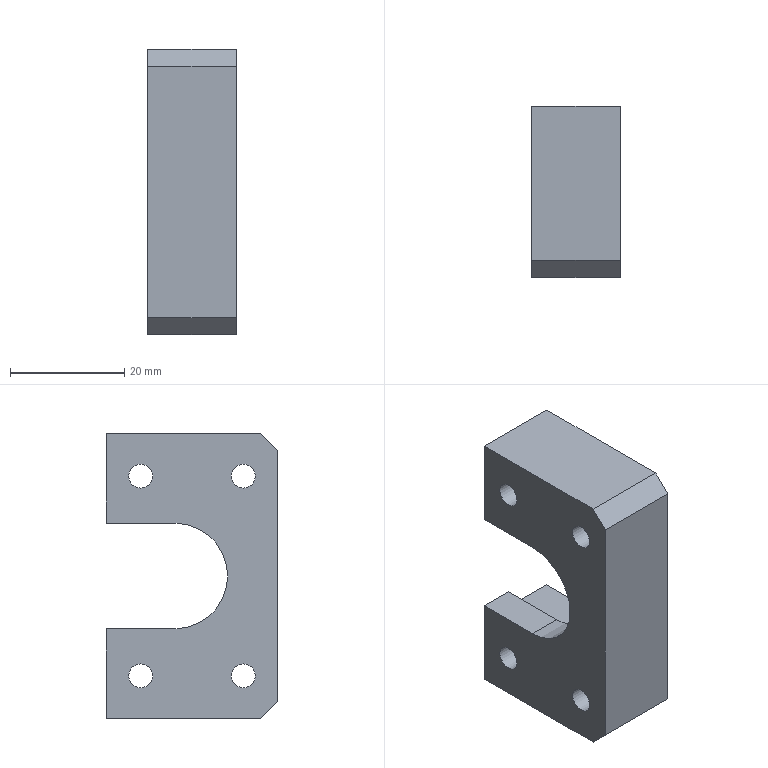Part | NX | 1 solid | 20 faces | box 15.5 x 30 x 50 mm | volume 14931 mm3 | plane 14 | cylinder 6 | commonest cylinder face diameters 4.2 x4 18.5 x1 25 x1
STEP:
#1=CARTESIAN_POINT('',(6.,3.,-9.25));
#2=VERTEX_POINT('',#1);
#3=CARTESIAN_POINT('',(6.,3.,9.25));
#4=VERTEX_POINT('',#3);
#5=CARTESIAN_POINT('',(6.,3.,0.));
#6=DIRECTION('',(1.,0.,0.));
#7=DIRECTION('',(0.,0.,-1.));
#8=AXIS2_PLACEMENT_3D('',#5,#6,#7);
#9=CIRCLE('',#8,9.25);
#10=EDGE_CURVE('',#2,#4,#9,.F.);
#11=ORIENTED_EDGE('',*,*,#10,.F.);
#12=CARTESIAN_POINT('',(0.,3.,-9.25));
#13=VERTEX_POINT('',#12);
#14=CARTESIAN_POINT('',(-4.5,3.,-9.25));
#15=DIRECTION('',(1.,0.,0.));
#16=VECTOR('',#15,1000.);
#17=LINE('',#14,#16);
#18=EDGE_CURVE('',#13,#2,#17,.T.);
#19=ORIENTED_EDGE('',*,*,#18,.F.);
#20=CARTESIAN_POINT('',(0.,3.,9.25));
#21=VERTEX_POINT('',#20);
#22=CARTESIAN_POINT('',(0.,3.,0.));
#23=DIRECTION('',(1.,0.,0.));
#24=DIRECTION('',(0.,0.,-1.));
#25=AXIS2_PLACEMENT_3D('',#22,#23,#24);
#26=CIRCLE('',#25,9.25);
#27=EDGE_CURVE('',#21,#13,#26,.T.);
#28=ORIENTED_EDGE('',*,*,#27,.F.);
#29=CARTESIAN_POINT('',(-4.5,3.,9.25));
#30=DIRECTION('',(1.,0.,0.));
#31=VECTOR('',#30,1000.);
#32=LINE('',#29,#31);
#33=EDGE_CURVE('',#21,#4,#32,.T.);
#34=ORIENTED_EDGE('',*,*,#33,.T.);
#35=EDGE_LOOP('',(#11,#19,#28,#34));
#36=FACE_BOUND('',#35,.T.);
#37=CARTESIAN_POINT('',(-4.5,3.,0.));
#38=DIRECTION('',(1.,0.,0.));
#39=DIRECTION('',(0.,0.,-1.));
#40=AXIS2_PLACEMENT_3D('',#37,#38,#39);
#41=CYLINDRICAL_SURFACE('',#40,9.25);
#42=ADVANCED_FACE('',(#36),#41,.F.);
#43=CARTESIAN_POINT('',(6.,15.,9.25));
#44=VERTEX_POINT('',#43);
#45=CARTESIAN_POINT('',(6.,3.,9.25));
#46=DIRECTION('',(0.,1.,0.));
#47=VECTOR('',#46,1000.);
#48=LINE('',#45,#47);
#49=EDGE_CURVE('',#4,#44,#48,.T.);
#50=ORIENTED_EDGE('',*,*,#49,.F.);
#51=ORIENTED_EDGE('',*,*,#33,.F.);
#52=CARTESIAN_POINT('',(0.,15.,9.25));
#53=VERTEX_POINT('',#52);
#54=CARTESIAN_POINT('',(0.,0.,9.25));
#55=DIRECTION('',(0.,-1.,0.));
#56=VECTOR('',#55,1000.);
#57=LINE('',#54,#56);
#58=EDGE_CURVE('',#53,#21,#57,.T.);
#59=ORIENTED_EDGE('',*,*,#58,.F.);
#60=CARTESIAN_POINT('',(15.5,15.,9.25));
#61=DIRECTION('',(-1.,0.,0.));
#62=VECTOR('',#61,1000.);
#63=LINE('',#60,#62);
#64=EDGE_CURVE('',#44,#53,#63,.T.);
#65=ORIENTED_EDGE('',*,*,#64,.F.);
#66=EDGE_LOOP('',(#50,#51,#59,#65));
#67=FACE_BOUND('',#66,.T.);
#68=CARTESIAN_POINT('',(-4.5,3.,9.25));
#69=DIRECTION('',(0.,0.,1.));
#70=DIRECTION('',(0.,-1.,0.));
#71=AXIS2_PLACEMENT_3D('',#68,#69,#70);
#72=PLANE('',#71);
#73=ADVANCED_FACE('',(#67),#72,.F.);
#74=CARTESIAN_POINT('',(6.,15.,-9.25));
#75=VERTEX_POINT('',#74);
#76=CARTESIAN_POINT('',(6.,3.,-9.25));
#77=DIRECTION('',(0.,-1.,0.));
#78=VECTOR('',#77,1000.);
#79=LINE('',#76,#78);
#80=EDGE_CURVE('',#75,#2,#79,.T.);
#81=ORIENTED_EDGE('',*,*,#80,.F.);
#82=CARTESIAN_POINT('',(0.,15.,-9.25));
#83=VERTEX_POINT('',#82);
#84=CARTESIAN_POINT('',(15.5,15.,-9.25));
#85=DIRECTION('',(1.,0.,0.));
#86=VECTOR('',#85,1000.);
#87=LINE('',#84,#86);
#88=EDGE_CURVE('',#83,#75,#87,.T.);
#89=ORIENTED_EDGE('',*,*,#88,.F.);
#90=CARTESIAN_POINT('',(0.,0.,-9.25));
#91=DIRECTION('',(0.,1.,0.));
#92=VECTOR('',#91,1000.);
#93=LINE('',#90,#92);
#94=EDGE_CURVE('',#13,#83,#93,.T.);
#95=ORIENTED_EDGE('',*,*,#94,.F.);
#96=ORIENTED_EDGE('',*,*,#18,.T.);
#97=EDGE_LOOP('',(#81,#89,#95,#96));
#98=FACE_BOUND('',#97,.T.);
#99=CARTESIAN_POINT('',(-4.5,3.,-9.25));
#100=DIRECTION('',(0.,0.,-1.));
#101=DIRECTION('',(0.,1.,0.));
#102=AXIS2_PLACEMENT_3D('',#99,#100,#101);
#103=PLANE('',#102);
#104=ADVANCED_FACE('',(#98),#103,.F.);
#105=CARTESIAN_POINT('',(15.5,15.,12.5));
#106=VERTEX_POINT('',#105);
#107=CARTESIAN_POINT('',(15.5,15.,25.));
#108=VERTEX_POINT('',#107);
#109=CARTESIAN_POINT('',(15.5,15.,25.));
#110=DIRECTION('',(0.,0.,1.));
#111=VECTOR('',#110,1000.);
#112=LINE('',#109,#111);
#113=EDGE_CURVE('',#106,#108,#112,.T.);
#114=ORIENTED_EDGE('',*,*,#113,.F.);
#115=CARTESIAN_POINT('',(6.,15.,12.5));
#116=VERTEX_POINT('',#115);
#117=CARTESIAN_POINT('',(6.,15.,12.5));
#118=DIRECTION('',(1.,0.,0.));
#119=VECTOR('',#118,1000.);
#120=LINE('',#117,#119);
#121=EDGE_CURVE('',#116,#106,#120,.T.);
#122=ORIENTED_EDGE('',*,*,#121,.F.);
#123=CARTESIAN_POINT('',(6.,15.,25.));
#124=DIRECTION('',(0.,0.,1.));
#125=VECTOR('',#124,1000.);
#126=LINE('',#123,#125);
#127=EDGE_CURVE('',#44,#116,#126,.T.);
#128=ORIENTED_EDGE('',*,*,#127,.F.);
#129=ORIENTED_EDGE('',*,*,#64,.T.);
#130=CARTESIAN_POINT('',(0.,15.,25.));
#131=VERTEX_POINT('',#130);
#132=CARTESIAN_POINT('',(0.,15.,25.));
#133=DIRECTION('',(0.,0.,1.));
#134=VECTOR('',#133,1000.);
#135=LINE('',#132,#134);
#136=EDGE_CURVE('',#53,#131,#135,.T.);
#137=ORIENTED_EDGE('',*,*,#136,.T.);
#138=CARTESIAN_POINT('',(15.5,15.,25.));
#139=DIRECTION('',(-1.,0.,0.));
#140=VECTOR('',#139,1000.);
#141=LINE('',#138,#140);
#142=EDGE_CURVE('',#108,#131,#141,.T.);
#143=ORIENTED_EDGE('',*,*,#142,.F.);
#144=EDGE_LOOP('',(#114,#122,#128,#129,#137,#143));
#145=FACE_BOUND('',#144,.T.);
#146=CARTESIAN_POINT('',(15.5,15.,25.));
#147=DIRECTION('',(0.,-1.,0.));
#148=DIRECTION('',(0.,0.,-1.));
#149=AXIS2_PLACEMENT_3D('',#146,#147,#148);
#150=PLANE('',#149);
#151=ADVANCED_FACE('',(#145),#150,.F.);
#152=CARTESIAN_POINT('',(15.5,-12.,-25.));
#153=VERTEX_POINT('',#152);
#154=CARTESIAN_POINT('',(15.5,15.,-25.));
#155=VERTEX_POINT('',#154);
#156=CARTESIAN_POINT('',(15.5,15.,-25.));
#157=DIRECTION('',(0.,1.,0.));
#158=VECTOR('',#157,1000.);
#159=LINE('',#156,#158);
#160=EDGE_CURVE('',#153,#155,#159,.T.);
#161=ORIENTED_EDGE('',*,*,#160,.F.);
#162=CARTESIAN_POINT('',(0.,-12.,-25.));
#163=VERTEX_POINT('',#162);
#164=CARTESIAN_POINT('',(15.5,-12.,-25.));
#165=DIRECTION('',(-1.,0.,0.));
#166=VECTOR('',#165,1000.);
#167=LINE('',#164,#166);
#168=EDGE_CURVE('',#153,#163,#167,.T.);
#169=ORIENTED_EDGE('',*,*,#168,.T.);
#170=CARTESIAN_POINT('',(0.,15.,-25.));
#171=VERTEX_POINT('',#170);
#172=CARTESIAN_POINT('',(0.,15.,-25.));
#173=DIRECTION('',(0.,1.,0.));
#174=VECTOR('',#173,1000.);
#175=LINE('',#172,#174);
#176=EDGE_CURVE('',#163,#171,#175,.T.);
#177=ORIENTED_EDGE('',*,*,#176,.T.);
#178=CARTESIAN_POINT('',(15.5,15.,-25.));
#179=DIRECTION('',(-1.,0.,0.));
#180=VECTOR('',#179,1000.);
#181=LINE('',#178,#180);
#182=EDGE_CURVE('',#155,#171,#181,.T.);
#183=ORIENTED_EDGE('',*,*,#182,.F.);
#184=EDGE_LOOP('',(#161,#169,#177,#183));
#185=FACE_BOUND('',#184,.T.);
#186=CARTESIAN_POINT('',(15.5,15.,-25.));
#187=DIRECTION('',(0.,0.,1.));
#188=DIRECTION('',(0.,-1.,0.));
#189=AXIS2_PLACEMENT_3D('',#186,#187,#188);
#190=PLANE('',#189);
#191=ADVANCED_FACE('',(#185),#190,.F.);
#192=CARTESIAN_POINT('',(6.,15.,-12.5));
#193=VERTEX_POINT('',#192);
#194=CARTESIAN_POINT('',(6.,15.,25.));
#195=DIRECTION('',(0.,0.,1.));
#196=VECTOR('',#195,1000.);
#197=LINE('',#194,#196);
#198=EDGE_CURVE('',#193,#75,#197,.T.);
#199=ORIENTED_EDGE('',*,*,#198,.F.);
#200=CARTESIAN_POINT('',(15.5,15.,-12.5));
#201=VERTEX_POINT('',#200);
#202=CARTESIAN_POINT('',(6.,15.,-12.5));
#203=DIRECTION('',(1.,0.,0.));
#204=VECTOR('',#203,1000.);
#205=LINE('',#202,#204);
#206=EDGE_CURVE('',#193,#201,#205,.T.);
#207=ORIENTED_EDGE('',*,*,#206,.T.);
#208=CARTESIAN_POINT('',(15.5,15.,25.));
#209=DIRECTION('',(0.,0.,1.));
#210=VECTOR('',#209,1000.);
#211=LINE('',#208,#210);
#212=EDGE_CURVE('',#155,#201,#211,.T.);
#213=ORIENTED_EDGE('',*,*,#212,.F.);
#214=ORIENTED_EDGE('',*,*,#182,.T.);
#215=CARTESIAN_POINT('',(0.,15.,25.));
#216=DIRECTION('',(0.,0.,1.));
#217=VECTOR('',#216,1000.);
#218=LINE('',#215,#217);
#219=EDGE_CURVE('',#171,#83,#218,.T.);
#220=ORIENTED_EDGE('',*,*,#219,.T.);
#221=ORIENTED_EDGE('',*,*,#88,.T.);
#222=EDGE_LOOP('',(#199,#207,#213,#214,#220,#221));
#223=FACE_BOUND('',#222,.T.);
#224=CARTESIAN_POINT('',(15.5,15.,25.));
#225=DIRECTION('',(0.,-1.,0.));
#226=DIRECTION('',(0.,0.,-1.));
#227=AXIS2_PLACEMENT_3D('',#224,#225,#226);
#228=PLANE('',#227);
#229=ADVANCED_FACE('',(#223),#228,.F.);
#230=CARTESIAN_POINT('',(0.,-12.,25.));
#231=VERTEX_POINT('',#230);
#232=CARTESIAN_POINT('',(0.,15.,25.));
#233=DIRECTION('',(0.,-1.,0.));
#234=VECTOR('',#233,1000.);
#235=LINE('',#232,#234);
#236=EDGE_CURVE('',#131,#231,#235,.T.);
#237=ORIENTED_EDGE('',*,*,#236,.T.);
#238=CARTESIAN_POINT('',(15.5,-12.,25.));
#239=VERTEX_POINT('',#238);
#240=CARTESIAN_POINT('',(15.5,-12.,25.));
#241=DIRECTION('',(1.,0.,0.));
#242=VECTOR('',#241,1000.);
#243=LINE('',#240,#242);
#244=EDGE_CURVE('',#231,#239,#243,.T.);
#245=ORIENTED_EDGE('',*,*,#244,.T.);
#246=CARTESIAN_POINT('',(15.5,15.,25.));
#247=DIRECTION('',(0.,-1.,0.));
#248=VECTOR('',#247,1000.);
#249=LINE('',#246,#248);
#250=EDGE_CURVE('',#108,#239,#249,.T.);
#251=ORIENTED_EDGE('',*,*,#250,.F.);
#252=ORIENTED_EDGE('',*,*,#142,.T.);
#253=EDGE_LOOP('',(#237,#245,#251,#252));
#254=FACE_BOUND('',#253,.T.);
#255=CARTESIAN_POINT('',(15.5,15.,25.));
#256=DIRECTION('',(0.,0.,-1.));
#257=DIRECTION('',(0.,1.,0.));
#258=AXIS2_PLACEMENT_3D('',#255,#256,#257);
#259=PLANE('',#258);
#260=ADVANCED_FACE('',(#254),#259,.F.);
#261=CARTESIAN_POINT('',(15.5,-15.,22.));
#262=VERTEX_POINT('',#261);
#263=CARTESIAN_POINT('',(15.5,-15.,-22.));
#264=VERTEX_POINT('',#263);
#265=CARTESIAN_POINT('',(15.5,-15.,25.));
#266=DIRECTION('',(0.,0.,-1.));
#267=VECTOR('',#266,1000.);
#268=LINE('',#265,#267);
#269=EDGE_CURVE('',#262,#264,#268,.T.);
#270=ORIENTED_EDGE('',*,*,#269,.F.);
#271=CARTESIAN_POINT('',(0.,-15.,22.));
#272=VERTEX_POINT('',#271);
#273=CARTESIAN_POINT('',(15.5,-15.,22.));
#274=DIRECTION('',(-1.,0.,0.));
#275=VECTOR('',#274,1000.);
#276=LINE('',#273,#275);
#277=EDGE_CURVE('',#262,#272,#276,.T.);
#278=ORIENTED_EDGE('',*,*,#277,.T.);
#279=CARTESIAN_POINT('',(0.,-15.,-22.));
#280=VERTEX_POINT('',#279);
#281=CARTESIAN_POINT('',(0.,-15.,25.));
#282=DIRECTION('',(0.,0.,-1.));
#283=VECTOR('',#282,1000.);
#284=LINE('',#281,#283);
#285=EDGE_CURVE('',#272,#280,#284,.T.);
#286=ORIENTED_EDGE('',*,*,#285,.T.);
#287=CARTESIAN_POINT('',(15.5,-15.,-22.));
#288=DIRECTION('',(1.,0.,0.));
#289=VECTOR('',#288,1000.);
#290=LINE('',#287,#289);
#291=EDGE_CURVE('',#280,#264,#290,.T.);
#292=ORIENTED_EDGE('',*,*,#291,.T.);
#293=EDGE_LOOP('',(#270,#278,#286,#292));
#294=FACE_BOUND('',#293,.T.);
#295=CARTESIAN_POINT('',(15.5,-15.,25.));
#296=DIRECTION('',(0.,1.,0.));
#297=DIRECTION('',(0.,0.,1.));
#298=AXIS2_PLACEMENT_3D('',#295,#296,#297);
#299=PLANE('',#298);
#300=ADVANCED_FACE('',(#294),#299,.F.);
#301=CARTESIAN_POINT('',(15.5,9.,-15.4));
#302=VERTEX_POINT('',#301);
#303=CARTESIAN_POINT('',(15.5,9.,-17.5));
#304=DIRECTION('',(-1.,0.,0.));
#305=DIRECTION('',(0.,0.,1.));
#306=AXIS2_PLACEMENT_3D('',#303,#304,#305);
#307=CIRCLE('',#306,2.1);
#308=EDGE_CURVE('',#302,#302,#307,.T.);
#309=ORIENTED_EDGE('',*,*,#308,.T.);
#310=EDGE_LOOP('',(#309));
#311=FACE_BOUND('',#310,.T.);
#312=CARTESIAN_POINT('',(15.5,-9.,-15.4));
#313=VERTEX_POINT('',#312);
#314=CARTESIAN_POINT('',(15.5,-9.,-17.5));
#315=DIRECTION('',(-1.,0.,0.));
#316=DIRECTION('',(0.,0.,1.));
#317=AXIS2_PLACEMENT_3D('',#314,#315,#316);
#318=CIRCLE('',#317,2.1);
#319=EDGE_CURVE('',#313,#313,#318,.T.);
#320=ORIENTED_EDGE('',*,*,#319,.T.);
#321=EDGE_LOOP('',(#320));
#322=FACE_BOUND('',#321,.T.);
#323=CARTESIAN_POINT('',(15.5,9.,19.6));
#324=VERTEX_POINT('',#323);
#325=CARTESIAN_POINT('',(15.5,9.,17.5));
#326=DIRECTION('',(-1.,0.,0.));
#327=DIRECTION('',(0.,0.,1.));
#328=AXIS2_PLACEMENT_3D('',#325,#326,#327);
#329=CIRCLE('',#328,2.1);
#330=EDGE_CURVE('',#324,#324,#329,.T.);
#331=ORIENTED_EDGE('',*,*,#330,.T.);
#332=EDGE_LOOP('',(#331));
#333=FACE_BOUND('',#332,.T.);
#334=CARTESIAN_POINT('',(15.5,-9.,19.6));
#335=VERTEX_POINT('',#334);
#336=CARTESIAN_POINT('',(15.5,-9.,17.5));
#337=DIRECTION('',(-1.,0.,0.));
#338=DIRECTION('',(0.,0.,1.));
#339=AXIS2_PLACEMENT_3D('',#336,#337,#338);
#340=CIRCLE('',#339,2.1);
#341=EDGE_CURVE('',#335,#335,#340,.T.);
#342=ORIENTED_EDGE('',*,*,#341,.T.);
#343=EDGE_LOOP('',(#342));
#344=FACE_BOUND('',#343,.T.);
#345=CARTESIAN_POINT('',(15.5,3.,12.5));
#346=VERTEX_POINT('',#345);
#347=CARTESIAN_POINT('',(15.5,3.,12.5));
#348=DIRECTION('',(0.,-1.,0.));
#349=VECTOR('',#348,1000.);
#350=LINE('',#347,#349);
#351=EDGE_CURVE('',#106,#346,#350,.T.);
#352=ORIENTED_EDGE('',*,*,#351,.F.);
#353=ORIENTED_EDGE('',*,*,#113,.T.);
#354=ORIENTED_EDGE('',*,*,#250,.T.);
#355=CARTESIAN_POINT('',(15.5,-18.5,18.5));
#356=DIRECTION('',(0.,0.7071,0.7071));
#357=VECTOR('',#356,1000.);
#358=LINE('',#355,#357);
#359=EDGE_CURVE('',#239,#262,#358,.F.);
#360=ORIENTED_EDGE('',*,*,#359,.T.);
#361=ORIENTED_EDGE('',*,*,#269,.T.);
#362=CARTESIAN_POINT('',(15.5,-18.5,-18.5));
#363=DIRECTION('',(0.,-0.7071,0.7071));
#364=VECTOR('',#363,1000.);
#365=LINE('',#362,#364);
#366=EDGE_CURVE('',#264,#153,#365,.F.);
#367=ORIENTED_EDGE('',*,*,#366,.T.);
#368=ORIENTED_EDGE('',*,*,#160,.T.);
#369=ORIENTED_EDGE('',*,*,#212,.T.);
#370=CARTESIAN_POINT('',(15.5,3.,-12.5));
#371=VERTEX_POINT('',#370);
#372=CARTESIAN_POINT('',(15.5,3.,-12.5));
#373=DIRECTION('',(0.,1.,0.));
#374=VECTOR('',#373,1000.);
#375=LINE('',#372,#374);
#376=EDGE_CURVE('',#371,#201,#375,.T.);
#377=ORIENTED_EDGE('',*,*,#376,.F.);
#378=CARTESIAN_POINT('',(15.5,3.,0.));
#379=DIRECTION('',(1.,0.,0.));
#380=DIRECTION('',(0.,0.,-1.));
#381=AXIS2_PLACEMENT_3D('',#378,#379,#380);
#382=CIRCLE('',#381,12.5);
#383=EDGE_CURVE('',#346,#371,#382,.T.);
#384=ORIENTED_EDGE('',*,*,#383,.F.);
#385=EDGE_LOOP('',(#352,#353,#354,#360,#361,#367,#368,#369,#377,#384));
#386=FACE_BOUND('',#385,.T.);
#387=CARTESIAN_POINT('',(15.5,0.,0.));
#388=DIRECTION('',(1.,0.,0.));
#389=DIRECTION('',(0.,0.,-1.));
#390=AXIS2_PLACEMENT_3D('',#387,#388,#389);
#391=PLANE('',#390);
#392=ADVANCED_FACE('',(#311,#322,#333,#344,#386),#391,.T.);
#393=CARTESIAN_POINT('',(0.,9.,-15.4));
#394=VERTEX_POINT('',#393);
#395=CARTESIAN_POINT('',(0.,9.,-17.5));
#396=DIRECTION('',(-1.,0.,0.));
#397=DIRECTION('',(0.,0.,1.));
#398=AXIS2_PLACEMENT_3D('',#395,#396,#397);
#399=CIRCLE('',#398,2.1);
#400=EDGE_CURVE('',#394,#394,#399,.T.);
#401=ORIENTED_EDGE('',*,*,#400,.F.);
#402=EDGE_LOOP('',(#401));
#403=FACE_BOUND('',#402,.T.);
#404=CARTESIAN_POINT('',(0.,-9.,-15.4));
#405=VERTEX_POINT('',#404);
#406=CARTESIAN_POINT('',(0.,-9.,-17.5));
#407=DIRECTION('',(-1.,0.,0.));
#408=DIRECTION('',(0.,0.,1.));
#409=AXIS2_PLACEMENT_3D('',#406,#407,#408);
#410=CIRCLE('',#409,2.1);
#411=EDGE_CURVE('',#405,#405,#410,.T.);
#412=ORIENTED_EDGE('',*,*,#411,.F.);
#413=EDGE_LOOP('',(#412));
#414=FACE_BOUND('',#413,.T.);
#415=CARTESIAN_POINT('',(0.,9.,19.6));
#416=VERTEX_POINT('',#415);
#417=CARTESIAN_POINT('',(0.,9.,17.5));
#418=DIRECTION('',(-1.,0.,0.));
#419=DIRECTION('',(0.,0.,1.));
#420=AXIS2_PLACEMENT_3D('',#417,#418,#419);
#421=CIRCLE('',#420,2.1);
#422=EDGE_CURVE('',#416,#416,#421,.T.);
#423=ORIENTED_EDGE('',*,*,#422,.F.);
#424=EDGE_LOOP('',(#423));
#425=FACE_BOUND('',#424,.T.);
#426=CARTESIAN_POINT('',(0.,-9.,19.6));
#427=VERTEX_POINT('',#426);
#428=CARTESIAN_POINT('',(0.,-9.,17.5));
#429=DIRECTION('',(-1.,0.,0.));
#430=DIRECTION('',(0.,0.,1.));
#431=AXIS2_PLACEMENT_3D('',#428,#429,#430);
#432=CIRCLE('',#431,2.1);
#433=EDGE_CURVE('',#427,#427,#432,.T.);
#434=ORIENTED_EDGE('',*,*,#433,.F.);
#435=EDGE_LOOP('',(#434));
#436=FACE_BOUND('',#435,.T.);
#437=ORIENTED_EDGE('',*,*,#285,.F.);
#438=CARTESIAN_POINT('',(0.,-15.,22.));
#439=DIRECTION('',(0.,-0.7071,-0.7071));
#440=VECTOR('',#439,1000.);
#441=LINE('',#438,#440);
#442=EDGE_CURVE('',#272,#231,#441,.F.);
#443=ORIENTED_EDGE('',*,*,#442,.T.);
#444=ORIENTED_EDGE('',*,*,#236,.F.);
#445=ORIENTED_EDGE('',*,*,#136,.F.);
#446=ORIENTED_EDGE('',*,*,#58,.T.);
#447=ORIENTED_EDGE('',*,*,#27,.T.);
#448=ORIENTED_EDGE('',*,*,#94,.T.);
#449=ORIENTED_EDGE('',*,*,#219,.F.);
#450=ORIENTED_EDGE('',*,*,#176,.F.);
#451=CARTESIAN_POINT('',(0.,-12.,-25.));
#452=DIRECTION('',(0.,0.7071,-0.7071));
#453=VECTOR('',#452,1000.);
#454=LINE('',#451,#453);
#455=EDGE_CURVE('',#163,#280,#454,.F.);
#456=ORIENTED_EDGE('',*,*,#455,.T.);
#457=EDGE_LOOP('',(#437,#443,#444,#445,#446,#447,#448,#449,#450,#456));
#458=FACE_BOUND('',#457,.T.);
#459=CARTESIAN_POINT('',(0.,0.,0.));
#460=DIRECTION('',(1.,0.,0.));
#461=DIRECTION('',(0.,0.,-1.));
#462=AXIS2_PLACEMENT_3D('',#459,#460,#461);
#463=PLANE('',#462);
#464=ADVANCED_FACE('',(#403,#414,#425,#436,#458),#463,.F.);
#465=ORIENTED_EDGE('',*,*,#359,.F.);
#466=ORIENTED_EDGE('',*,*,#244,.F.);
#467=ORIENTED_EDGE('',*,*,#442,.F.);
#468=ORIENTED_EDGE('',*,*,#277,.F.);
#469=EDGE_LOOP('',(#465,#466,#467,#468));
#470=FACE_BOUND('',#469,.T.);
#471=CARTESIAN_POINT('',(15.5,-15.,22.));
#472=DIRECTION('',(0.,0.7071,-0.7071));
#473=DIRECTION('',(-1.,0.,0.));
#474=AXIS2_PLACEMENT_3D('',#471,#472,#473);
#475=PLANE('',#474);
#476=ADVANCED_FACE('',(#470),#475,.F.);
#477=ORIENTED_EDGE('',*,*,#366,.F.);
#478=ORIENTED_EDGE('',*,*,#291,.F.);
#479=ORIENTED_EDGE('',*,*,#455,.F.);
#480=ORIENTED_EDGE('',*,*,#168,.F.);
#481=EDGE_LOOP('',(#477,#478,#479,#480));
#482=FACE_BOUND('',#481,.T.);
#483=CARTESIAN_POINT('',(15.5,-12.,-25.));
#484=DIRECTION('',(0.,0.7071,0.7071));
#485=DIRECTION('',(-1.,0.,0.));
#486=AXIS2_PLACEMENT_3D('',#483,#484,#485);
#487=PLANE('',#486);
#488=ADVANCED_FACE('',(#482),#487,.F.);
#489=ORIENTED_EDGE('',*,*,#127,.T.);
#490=CARTESIAN_POINT('',(6.,3.,12.5));
#491=VERTEX_POINT('',#490);
#492=CARTESIAN_POINT('',(6.,3.,12.5));
#493=DIRECTION('',(0.,-1.,0.));
#494=VECTOR('',#493,1000.);
#495=LINE('',#492,#494);
#496=EDGE_CURVE('',#116,#491,#495,.T.);
#497=ORIENTED_EDGE('',*,*,#496,.T.);
#498=CARTESIAN_POINT('',(6.,3.,-12.5));
#499=VERTEX_POINT('',#498);
#500=CARTESIAN_POINT('',(6.,3.,0.));
#501=DIRECTION('',(1.,0.,0.));
#502=DIRECTION('',(0.,0.,-1.));
#503=AXIS2_PLACEMENT_3D('',#500,#501,#502);
#504=CIRCLE('',#503,12.5);
#505=EDGE_CURVE('',#491,#499,#504,.T.);
#506=ORIENTED_EDGE('',*,*,#505,.T.);
#507=CARTESIAN_POINT('',(6.,3.,-12.5));
#508=DIRECTION('',(0.,1.,0.));
#509=VECTOR('',#508,1000.);
#510=LINE('',#507,#509);
#511=EDGE_CURVE('',#499,#193,#510,.T.);
#512=ORIENTED_EDGE('',*,*,#511,.T.);
#513=ORIENTED_EDGE('',*,*,#198,.T.);
#514=ORIENTED_EDGE('',*,*,#80,.T.);
#515=ORIENTED_EDGE('',*,*,#10,.T.);
#516=ORIENTED_EDGE('',*,*,#49,.T.);
#517=EDGE_LOOP('',(#489,#497,#506,#512,#513,#514,#515,#516));
#518=FACE_BOUND('',#517,.T.);
#519=CARTESIAN_POINT('',(6.,3.,0.));
#520=DIRECTION('',(1.,0.,0.));
#521=DIRECTION('',(0.,0.,-1.));
#522=AXIS2_PLACEMENT_3D('',#519,#520,#521);
#523=PLANE('',#522);
#524=ADVANCED_FACE('',(#518),#523,.T.);
#525=ORIENTED_EDGE('',*,*,#383,.T.);
#526=CARTESIAN_POINT('',(6.,3.,-12.5));
#527=DIRECTION('',(1.,0.,0.));
#528=VECTOR('',#527,1000.);
#529=LINE('',#526,#528);
#530=EDGE_CURVE('',#499,#371,#529,.T.);
#531=ORIENTED_EDGE('',*,*,#530,.F.);
#532=ORIENTED_EDGE('',*,*,#505,.F.);
#533=CARTESIAN_POINT('',(6.,3.,12.5));
#534=DIRECTION('',(1.,0.,0.));
#535=VECTOR('',#534,1000.);
#536=LINE('',#533,#535);
#537=EDGE_CURVE('',#491,#346,#536,.T.);
#538=ORIENTED_EDGE('',*,*,#537,.T.);
#539=EDGE_LOOP('',(#525,#531,#532,#538));
#540=FACE_BOUND('',#539,.T.);
#541=CARTESIAN_POINT('',(6.,3.,0.));
#542=DIRECTION('',(1.,0.,0.));
#543=DIRECTION('',(0.,0.,-1.));
#544=AXIS2_PLACEMENT_3D('',#541,#542,#543);
#545=CYLINDRICAL_SURFACE('',#544,12.5);
#546=ADVANCED_FACE('',(#540),#545,.F.);
#547=ORIENTED_EDGE('',*,*,#351,.T.);
#548=ORIENTED_EDGE('',*,*,#537,.F.);
#549=ORIENTED_EDGE('',*,*,#496,.F.);
#550=ORIENTED_EDGE('',*,*,#121,.T.);
#551=EDGE_LOOP('',(#547,#548,#549,#550));
#552=FACE_BOUND('',#551,.T.);
#553=CARTESIAN_POINT('',(6.,3.,12.5));
#554=DIRECTION('',(0.,0.,1.));
#555=DIRECTION('',(1.,0.,0.));
#556=AXIS2_PLACEMENT_3D('',#553,#554,#555);
#557=PLANE('',#556);
#558=ADVANCED_FACE('',(#552),#557,.F.);
#559=ORIENTED_EDGE('',*,*,#376,.T.);
#560=ORIENTED_EDGE('',*,*,#206,.F.);
#561=ORIENTED_EDGE('',*,*,#511,.F.);
#562=ORIENTED_EDGE('',*,*,#530,.T.);
#563=EDGE_LOOP('',(#559,#560,#561,#562));
#564=FACE_BOUND('',#563,.T.);
#565=CARTESIAN_POINT('',(6.,3.,-12.5));
#566=DIRECTION('',(0.,0.,-1.));
#567=DIRECTION('',(-1.,0.,0.));
#568=AXIS2_PLACEMENT_3D('',#565,#566,#567);
#569=PLANE('',#568);
#570=ADVANCED_FACE('',(#564),#569,.F.);
#571=ORIENTED_EDGE('',*,*,#341,.F.);
#572=EDGE_LOOP('',(#571));
#573=FACE_BOUND('',#572,.T.);
#574=ORIENTED_EDGE('',*,*,#433,.T.);
#575=EDGE_LOOP('',(#574));
#576=FACE_BOUND('',#575,.T.);
#577=CARTESIAN_POINT('',(0.,-9.,17.5));
#578=DIRECTION('',(-1.,0.,0.));
#579=DIRECTION('',(0.,0.,1.));
#580=AXIS2_PLACEMENT_3D('',#577,#578,#579);
#581=CYLINDRICAL_SURFACE('',#580,2.1);
#582=ADVANCED_FACE('',(#573,#576),#581,.F.);
#583=ORIENTED_EDGE('',*,*,#330,.F.);
#584=EDGE_LOOP('',(#583));
#585=FACE_BOUND('',#584,.T.);
#586=ORIENTED_EDGE('',*,*,#422,.T.);
#587=EDGE_LOOP('',(#586));
#588=FACE_BOUND('',#587,.T.);
#589=CARTESIAN_POINT('',(0.,9.,17.5));
#590=DIRECTION('',(-1.,0.,0.));
#591=DIRECTION('',(0.,0.,1.));
#592=AXIS2_PLACEMENT_3D('',#589,#590,#591);
#593=CYLINDRICAL_SURFACE('',#592,2.1);
#594=ADVANCED_FACE('',(#585,#588),#593,.F.);
#595=ORIENTED_EDGE('',*,*,#319,.F.);
#596=EDGE_LOOP('',(#595));
#597=FACE_BOUND('',#596,.T.);
#598=ORIENTED_EDGE('',*,*,#411,.T.);
#599=EDGE_LOOP('',(#598));
#600=FACE_BOUND('',#599,.T.);
#601=CARTESIAN_POINT('',(0.,-9.,-17.5));
#602=DIRECTION('',(-1.,0.,0.));
#603=DIRECTION('',(0.,0.,1.));
#604=AXIS2_PLACEMENT_3D('',#601,#602,#603);
#605=CYLINDRICAL_SURFACE('',#604,2.1);
#606=ADVANCED_FACE('',(#597,#600),#605,.F.);
#607=ORIENTED_EDGE('',*,*,#308,.F.);
#608=EDGE_LOOP('',(#607));
#609=FACE_BOUND('',#608,.T.);
#610=ORIENTED_EDGE('',*,*,#400,.T.);
#611=EDGE_LOOP('',(#610));
#612=FACE_BOUND('',#611,.T.);
#613=CARTESIAN_POINT('',(0.,9.,-17.5));
#614=DIRECTION('',(-1.,0.,0.));
#615=DIRECTION('',(0.,0.,1.));
#616=AXIS2_PLACEMENT_3D('',#613,#614,#615);
#617=CYLINDRICAL_SURFACE('',#616,2.1);
#618=ADVANCED_FACE('',(#609,#612),#617,.F.);
#619=CLOSED_SHELL('',(#42,#73,#104,#151,#191,#229,#260,#300,#392,#464,#476,#488,#524,#546,#558,#570,#582,#594,#606,#618));
#620=MANIFOLD_SOLID_BREP('',#619);
#621=(LENGTH_UNIT()NAMED_UNIT(*)SI_UNIT(.MILLI.,.METRE.));
#622=UNCERTAINTY_MEASURE_WITH_UNIT(LENGTH_MEASURE(0.00001),#621,'','');
#623=(NAMED_UNIT(*)PLANE_ANGLE_UNIT()SI_UNIT($,.RADIAN.));
#624=(NAMED_UNIT(*)SI_UNIT($,.STERADIAN.)SOLID_ANGLE_UNIT());
#625=(GEOMETRIC_REPRESENTATION_CONTEXT(3)GLOBAL_UNCERTAINTY_ASSIGNED_CONTEXT((#622))GLOBAL_UNIT_ASSIGNED_CONTEXT((#621,#623,#624))REPRESENTATION_CONTEXT('',''));
#626=ADVANCED_BREP_SHAPE_REPRESENTATION('',(#620),#625);